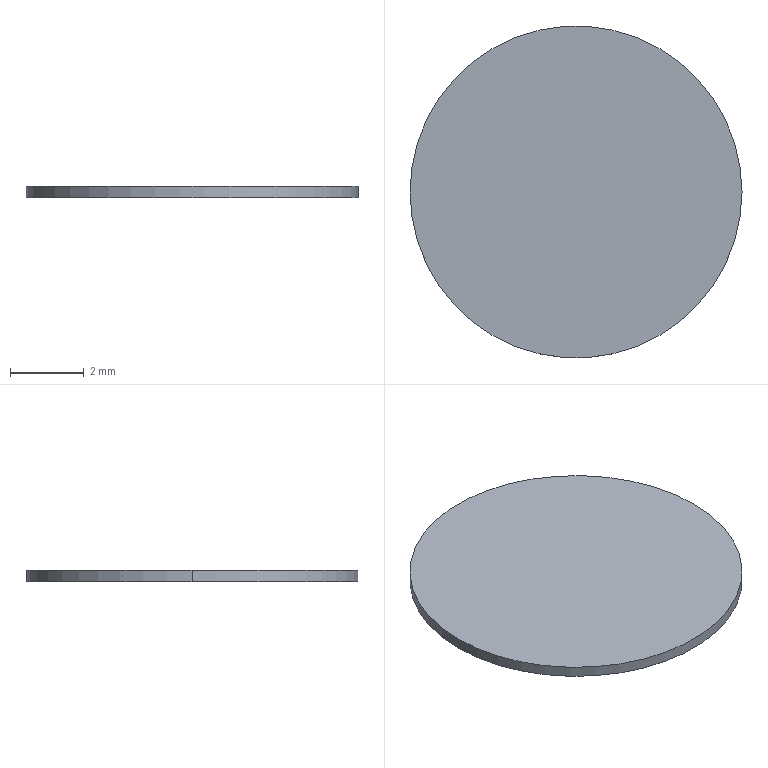Part | NX | features BREP 1 | 1 solid | 4 faces | box 9 x 9 x 0.3 mm | volume 19.085 mm3 | cylinder 2 | plane 2 | commonest cylinder face diameters 9 x2
STEP:
#1=CARTESIAN_POINT('',(4.5,0.,0.3));
#2=VERTEX_POINT('',#1);
#3=CARTESIAN_POINT('',(-4.5,0.,0.3));
#4=VERTEX_POINT('',#3);
#5=CARTESIAN_POINT('',(0.,0.,0.3));
#6=DIRECTION('',(0.,0.,1.));
#7=DIRECTION('',(-1.,0.,0.));
#8=AXIS2_PLACEMENT_3D('',#5,#6,#7);
#9=CIRCLE('',#8,4.5);
#10=EDGE_CURVE('',#2,#4,#9,.T.);
#11=ORIENTED_EDGE('',*,*,#10,.F.);
#12=CARTESIAN_POINT('',(4.5,0.,-0.000000001));
#13=VERTEX_POINT('',#12);
#14=CARTESIAN_POINT('',(4.5,0.,0.3));
#15=DIRECTION('',(0.,0.,1.));
#16=VECTOR('',#15,1000.);
#17=LINE('',#14,#16);
#18=EDGE_CURVE('',#13,#2,#17,.T.);
#19=ORIENTED_EDGE('',*,*,#18,.F.);
#20=CARTESIAN_POINT('',(-4.5,0.,-0.000000001));
#21=VERTEX_POINT('',#20);
#22=CARTESIAN_POINT('',(0.,0.,-0.000000001));
#23=DIRECTION('',(0.,0.,1.));
#24=DIRECTION('',(-1.,0.,0.));
#25=AXIS2_PLACEMENT_3D('',#22,#23,#24);
#26=CIRCLE('',#25,4.5);
#27=EDGE_CURVE('',#13,#21,#26,.T.);
#28=ORIENTED_EDGE('',*,*,#27,.T.);
#29=CARTESIAN_POINT('',(-4.5,0.,0.3));
#30=DIRECTION('',(0.,0.,1.));
#31=VECTOR('',#30,1000.);
#32=LINE('',#29,#31);
#33=EDGE_CURVE('',#21,#4,#32,.T.);
#34=ORIENTED_EDGE('',*,*,#33,.T.);
#35=EDGE_LOOP('',(#11,#19,#28,#34));
#36=FACE_BOUND('',#35,.T.);
#37=CARTESIAN_POINT('',(0.,0.,0.3));
#38=DIRECTION('',(0.,0.,-1.));
#39=DIRECTION('',(1.,0.,0.));
#40=AXIS2_PLACEMENT_3D('',#37,#38,#39);
#41=CYLINDRICAL_SURFACE('',#40,4.5);
#42=ADVANCED_FACE('',(#36),#41,.T.);
#43=CARTESIAN_POINT('',(0.,0.,0.3));
#44=DIRECTION('',(0.,0.,1.));
#45=DIRECTION('',(1.,0.,0.));
#46=AXIS2_PLACEMENT_3D('',#43,#44,#45);
#47=CIRCLE('',#46,4.5);
#48=EDGE_CURVE('',#4,#2,#47,.T.);
#49=ORIENTED_EDGE('',*,*,#48,.T.);
#50=ORIENTED_EDGE('',*,*,#10,.T.);
#51=EDGE_LOOP('',(#49,#50));
#52=FACE_BOUND('',#51,.T.);
#53=CARTESIAN_POINT('',(0.,0.,0.3));
#54=DIRECTION('',(0.,0.,1.));
#55=DIRECTION('',(-1.,0.,0.));
#56=AXIS2_PLACEMENT_3D('',#53,#54,#55);
#57=PLANE('',#56);
#58=ADVANCED_FACE('',(#52),#57,.T.);
#59=ORIENTED_EDGE('',*,*,#18,.T.);
#60=ORIENTED_EDGE('',*,*,#48,.F.);
#61=ORIENTED_EDGE('',*,*,#33,.F.);
#62=CARTESIAN_POINT('',(0.,0.,-0.000000001));
#63=DIRECTION('',(0.,0.,1.));
#64=DIRECTION('',(-1.,0.,0.));
#65=AXIS2_PLACEMENT_3D('',#62,#63,#64);
#66=CIRCLE('',#65,4.5);
#67=EDGE_CURVE('',#21,#13,#66,.T.);
#68=ORIENTED_EDGE('',*,*,#67,.T.);
#69=EDGE_LOOP('',(#59,#60,#61,#68));
#70=FACE_BOUND('',#69,.T.);
#71=CARTESIAN_POINT('',(0.,0.,0.3));
#72=DIRECTION('',(0.,0.,-1.));
#73=DIRECTION('',(-1.,0.,0.));
#74=AXIS2_PLACEMENT_3D('',#71,#72,#73);
#75=CYLINDRICAL_SURFACE('',#74,4.5);
#76=ADVANCED_FACE('',(#70),#75,.T.);
#77=ORIENTED_EDGE('',*,*,#67,.F.);
#78=ORIENTED_EDGE('',*,*,#27,.F.);
#79=EDGE_LOOP('',(#77,#78));
#80=FACE_BOUND('',#79,.T.);
#81=CARTESIAN_POINT('',(0.,0.,0.));
#82=DIRECTION('',(0.,0.,1.));
#83=DIRECTION('',(-1.,0.,0.));
#84=AXIS2_PLACEMENT_3D('',#81,#82,#83);
#85=PLANE('',#84);
#86=ADVANCED_FACE('',(#80),#85,.F.);
#87=CLOSED_SHELL('',(#42,#58,#76,#86));
#88=MANIFOLD_SOLID_BREP('',#87);
#89=(LENGTH_UNIT()NAMED_UNIT(*)SI_UNIT(.MILLI.,.METRE.));
#90=UNCERTAINTY_MEASURE_WITH_UNIT(LENGTH_MEASURE(0.00001),#89,'','');
#91=(NAMED_UNIT(*)PLANE_ANGLE_UNIT()SI_UNIT($,.RADIAN.));
#92=(NAMED_UNIT(*)SI_UNIT($,.STERADIAN.)SOLID_ANGLE_UNIT());
#93=(GEOMETRIC_REPRESENTATION_CONTEXT(3)GLOBAL_UNCERTAINTY_ASSIGNED_CONTEXT((#90))GLOBAL_UNIT_ASSIGNED_CONTEXT((#89,#91,#92))REPRESENTATION_CONTEXT('',''));
#94=ADVANCED_BREP_SHAPE_REPRESENTATION('',(#88),#93);